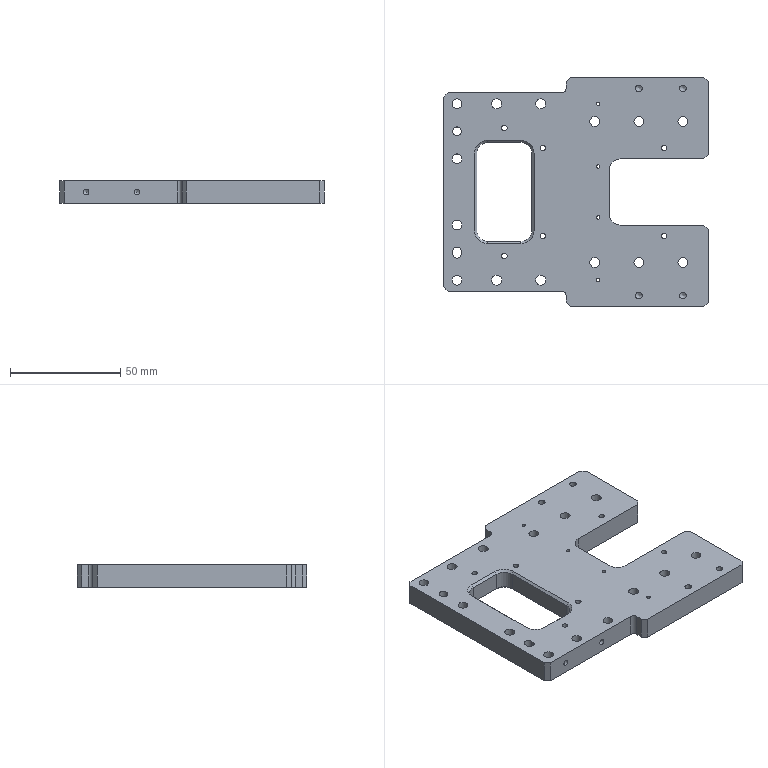Part | 1 solid | 123 faces | box 120 x 104 x 10 mm | volume 87014 mm3 | cylinder 57 | plane 50 | cone 16 | commonest cylinder face diameters 4.5 x14 8 x14 2.5 x10 10 x6 4 x5 1.6 x4